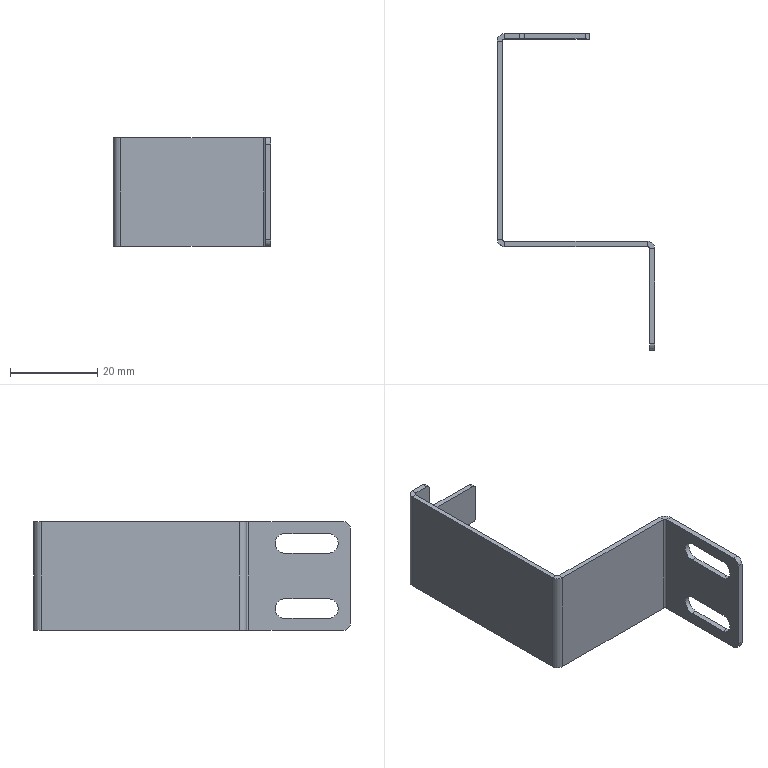Part | SolidWorks | features Fillet 2, FlatPattern 1, HoleWzd 1, ICE 1, SMBaseFlange 1, SheetMetal 1 | 1 solid | 48 faces | box 36.2 x 72.7 x 25 mm | volume 3370 mm3 | plane 32 | cylinder 16 | commonest cylinder face diameters 2 x4 4.5 x4 1 x3 3.4 x3 3 x2
STEP:
#1=CARTESIAN_POINT('',(0.,-20.,5.25));
#2=VERTEX_POINT('',#1);
#3=CARTESIAN_POINT('',(0.,-10.,5.25));
#4=VERTEX_POINT('',#3);
#5=CARTESIAN_POINT('',(0.,-20.,5.25));
#6=DIRECTION('',(0.,1.,0.));
#7=VECTOR('',#6,1000.);
#8=LINE('',#5,#7);
#9=EDGE_CURVE('',#2,#4,#8,.T.);
#10=ORIENTED_EDGE('',*,*,#9,.F.);
#11=CARTESIAN_POINT('',(0.,-20.,9.75));
#12=VERTEX_POINT('',#11);
#13=CARTESIAN_POINT('',(0.,-20.,7.5));
#14=DIRECTION('',(-1.,0.,0.));
#15=DIRECTION('',(0.,0.,1.));
#16=AXIS2_PLACEMENT_3D('',#13,#14,#15);
#17=CIRCLE('',#16,2.25);
#18=EDGE_CURVE('',#2,#12,#17,.T.);
#19=ORIENTED_EDGE('',*,*,#18,.T.);
#20=CARTESIAN_POINT('',(0.,-10.,9.75));
#21=VERTEX_POINT('',#20);
#22=CARTESIAN_POINT('',(0.,-20.,9.75));
#23=DIRECTION('',(0.,1.,0.));
#24=VECTOR('',#23,1000.);
#25=LINE('',#22,#24);
#26=EDGE_CURVE('',#12,#21,#25,.T.);
#27=ORIENTED_EDGE('',*,*,#26,.T.);
#28=CARTESIAN_POINT('',(0.,-10.,7.5));
#29=DIRECTION('',(-1.,0.,0.));
#30=DIRECTION('',(0.,0.,1.));
#31=AXIS2_PLACEMENT_3D('',#28,#29,#30);
#32=CIRCLE('',#31,2.25);
#33=EDGE_CURVE('',#21,#4,#32,.T.);
#34=ORIENTED_EDGE('',*,*,#33,.T.);
#35=EDGE_LOOP('',(#10,#19,#27,#34));
#36=FACE_BOUND('',#35,.T.);
#37=CARTESIAN_POINT('',(0.,-25.,11.));
#38=VERTEX_POINT('',#37);
#39=CARTESIAN_POINT('',(0.,-25.,-11.));
#40=VERTEX_POINT('',#39);
#41=CARTESIAN_POINT('',(0.,-25.,12.5));
#42=DIRECTION('',(0.,0.,-1.));
#43=VECTOR('',#42,1000.);
#44=LINE('',#41,#43);
#45=EDGE_CURVE('',#38,#40,#44,.T.);
#46=ORIENTED_EDGE('',*,*,#45,.T.);
#47=CARTESIAN_POINT('',(0.,-23.5,-12.5));
#48=VERTEX_POINT('',#47);
#49=CARTESIAN_POINT('',(0.,-23.5,-11.));
#50=DIRECTION('',(1.,0.,0.));
#51=DIRECTION('',(0.,0.,-1.));
#52=AXIS2_PLACEMENT_3D('',#49,#50,#51);
#53=CIRCLE('',#52,1.5);
#54=EDGE_CURVE('',#40,#48,#53,.T.);
#55=ORIENTED_EDGE('',*,*,#54,.T.);
#56=CARTESIAN_POINT('',(0.,-1.7,-12.5));
#57=VERTEX_POINT('',#56);
#58=CARTESIAN_POINT('',(0.,0.,-12.5));
#59=DIRECTION('',(0.,-1.,0.));
#60=VECTOR('',#59,1000.);
#61=LINE('',#58,#60);
#62=EDGE_CURVE('',#57,#48,#61,.T.);
#63=ORIENTED_EDGE('',*,*,#62,.F.);
#64=CARTESIAN_POINT('',(0.,-1.7,12.5));
#65=VERTEX_POINT('',#64);
#66=CARTESIAN_POINT('',(0.,-1.7,12.5));
#67=DIRECTION('',(0.,0.,-1.));
#68=VECTOR('',#67,1000.);
#69=LINE('',#66,#68);
#70=EDGE_CURVE('',#65,#57,#69,.T.);
#71=ORIENTED_EDGE('',*,*,#70,.F.);
#72=CARTESIAN_POINT('',(0.,-23.5,12.5));
#73=VERTEX_POINT('',#72);
#74=CARTESIAN_POINT('',(0.,0.,12.5));
#75=DIRECTION('',(0.,-1.,0.));
#76=VECTOR('',#75,1000.);
#77=LINE('',#74,#76);
#78=EDGE_CURVE('',#65,#73,#77,.T.);
#79=ORIENTED_EDGE('',*,*,#78,.T.);
#80=CARTESIAN_POINT('',(0.,-23.5,11.));
#81=DIRECTION('',(1.,0.,0.));
#82=DIRECTION('',(0.,0.,-1.));
#83=AXIS2_PLACEMENT_3D('',#80,#81,#82);
#84=CIRCLE('',#83,1.5);
#85=EDGE_CURVE('',#73,#38,#84,.T.);
#86=ORIENTED_EDGE('',*,*,#85,.T.);
#87=EDGE_LOOP('',(#46,#55,#63,#71,#79,#86));
#88=FACE_OUTER_BOUND('',#87,.T.);
#89=CARTESIAN_POINT('',(0.,-20.,-9.75));
#90=VERTEX_POINT('',#89);
#91=CARTESIAN_POINT('',(0.,-20.,-5.25));
#92=VERTEX_POINT('',#91);
#93=CARTESIAN_POINT('',(0.,-20.,-7.5));
#94=DIRECTION('',(-1.,0.,0.));
#95=DIRECTION('',(0.,0.,1.));
#96=AXIS2_PLACEMENT_3D('',#93,#94,#95);
#97=CIRCLE('',#96,2.25);
#98=EDGE_CURVE('',#90,#92,#97,.T.);
#99=ORIENTED_EDGE('',*,*,#98,.T.);
#100=CARTESIAN_POINT('',(0.,-10.,-5.25));
#101=VERTEX_POINT('',#100);
#102=CARTESIAN_POINT('',(0.,-20.,-5.25));
#103=DIRECTION('',(0.,1.,0.));
#104=VECTOR('',#103,1000.);
#105=LINE('',#102,#104);
#106=EDGE_CURVE('',#92,#101,#105,.T.);
#107=ORIENTED_EDGE('',*,*,#106,.T.);
#108=CARTESIAN_POINT('',(0.,-10.,-9.75));
#109=VERTEX_POINT('',#108);
#110=CARTESIAN_POINT('',(0.,-10.,-7.5));
#111=DIRECTION('',(-1.,0.,0.));
#112=DIRECTION('',(0.,0.,1.));
#113=AXIS2_PLACEMENT_3D('',#110,#111,#112);
#114=CIRCLE('',#113,2.25);
#115=EDGE_CURVE('',#101,#109,#114,.T.);
#116=ORIENTED_EDGE('',*,*,#115,.T.);
#117=CARTESIAN_POINT('',(0.,-20.,-9.75));
#118=DIRECTION('',(0.,1.,0.));
#119=VECTOR('',#118,1000.);
#120=LINE('',#117,#119);
#121=EDGE_CURVE('',#90,#109,#120,.T.);
#122=ORIENTED_EDGE('',*,*,#121,.F.);
#123=EDGE_LOOP('',(#99,#107,#116,#122));
#124=FACE_BOUND('',#123,.T.);
#125=CARTESIAN_POINT('',(0.,0.,12.5));
#126=DIRECTION('',(1.,0.,0.));
#127=DIRECTION('',(0.,0.,-1.));
#128=AXIS2_PLACEMENT_3D('',#125,#126,#127);
#129=PLANE('',#128);
#130=ADVANCED_FACE('',(#36,#88,#124),#129,.T.);
#131=CARTESIAN_POINT('',(-31.,47.7,-12.5));
#132=VERTEX_POINT('',#131);
#133=CARTESIAN_POINT('',(-34.5,47.7,-12.5));
#134=VERTEX_POINT('',#133);
#135=CARTESIAN_POINT('',(-35.,47.7,-12.5));
#136=DIRECTION('',(-1.,0.,0.));
#137=VECTOR('',#136,1000.);
#138=LINE('',#135,#137);
#139=EDGE_CURVE('',#132,#134,#138,.T.);
#140=ORIENTED_EDGE('',*,*,#139,.F.);
#141=CARTESIAN_POINT('',(-31.,46.5,-12.5));
#142=VERTEX_POINT('',#141);
#143=CARTESIAN_POINT('',(-31.,46.,-12.5));
#144=DIRECTION('',(0.,-1.,0.));
#145=VECTOR('',#144,1000.);
#146=LINE('',#143,#145);
#147=EDGE_CURVE('',#132,#142,#146,.T.);
#148=ORIENTED_EDGE('',*,*,#147,.T.);
#149=CARTESIAN_POINT('',(-34.5,46.5,-12.5));
#150=VERTEX_POINT('',#149);
#151=CARTESIAN_POINT('',(-35.,46.5,-12.5));
#152=DIRECTION('',(-1.,0.,0.));
#153=VECTOR('',#152,1000.);
#154=LINE('',#151,#153);
#155=EDGE_CURVE('',#142,#150,#154,.T.);
#156=ORIENTED_EDGE('',*,*,#155,.T.);
#157=CARTESIAN_POINT('',(-34.5,46.5,-12.5));
#158=DIRECTION('',(0.,1.,0.));
#159=VECTOR('',#158,1000.);
#160=LINE('',#157,#159);
#161=EDGE_CURVE('',#150,#134,#160,.T.);
#162=ORIENTED_EDGE('',*,*,#161,.T.);
#163=EDGE_LOOP('',(#140,#148,#156,#162));
#164=FACE_OUTER_BOUND('',#163,.T.);
#165=CARTESIAN_POINT('',(-36.2,46.,-12.5));
#166=DIRECTION('',(0.,0.,-1.));
#167=DIRECTION('',(-1.,0.,0.));
#168=AXIS2_PLACEMENT_3D('',#165,#166,#167);
#169=PLANE('',#168);
#170=ADVANCED_FACE('',(#164),#169,.T.);
#171=CARTESIAN_POINT('',(-30.,46.5,-5.));
#172=VERTEX_POINT('',#171);
#173=CARTESIAN_POINT('',(-16.,46.5,-5.));
#174=VERTEX_POINT('',#173);
#175=CARTESIAN_POINT('',(-30.,46.5,-5.));
#176=DIRECTION('',(1.,0.,0.));
#177=VECTOR('',#176,1000.);
#178=LINE('',#175,#177);
#179=EDGE_CURVE('',#172,#174,#178,.T.);
#180=ORIENTED_EDGE('',*,*,#179,.T.);
#181=CARTESIAN_POINT('',(-15.,46.5,-4.));
#182=VERTEX_POINT('',#181);
#183=CARTESIAN_POINT('',(-16.,46.5,-4.));
#184=DIRECTION('',(0.,-1.,0.));
#185=DIRECTION('',(0.,0.,-1.));
#186=AXIS2_PLACEMENT_3D('',#183,#184,#185);
#187=CIRCLE('',#186,1.);
#188=EDGE_CURVE('',#174,#182,#187,.T.);
#189=ORIENTED_EDGE('',*,*,#188,.T.);
#190=CARTESIAN_POINT('',(-15.,46.5,4.));
#191=VERTEX_POINT('',#190);
#192=CARTESIAN_POINT('',(-15.,46.5,12.5));
#193=DIRECTION('',(0.,0.,-1.));
#194=VECTOR('',#193,1000.);
#195=LINE('',#192,#194);
#196=EDGE_CURVE('',#191,#182,#195,.T.);
#197=ORIENTED_EDGE('',*,*,#196,.F.);
#198=CARTESIAN_POINT('',(-16.,46.5,5.));
#199=VERTEX_POINT('',#198);
#200=CARTESIAN_POINT('',(-16.,46.5,4.));
#201=DIRECTION('',(0.,-1.,0.));
#202=DIRECTION('',(0.,0.,-1.));
#203=AXIS2_PLACEMENT_3D('',#200,#201,#202);
#204=CIRCLE('',#203,1.);
#205=EDGE_CURVE('',#191,#199,#204,.T.);
#206=ORIENTED_EDGE('',*,*,#205,.T.);
#207=CARTESIAN_POINT('',(-30.,46.5,5.));
#208=VERTEX_POINT('',#207);
#209=CARTESIAN_POINT('',(-30.,46.5,5.));
#210=DIRECTION('',(-1.,0.,0.));
#211=VECTOR('',#210,1000.);
#212=LINE('',#209,#211);
#213=EDGE_CURVE('',#199,#208,#212,.T.);
#214=ORIENTED_EDGE('',*,*,#213,.T.);
#215=CARTESIAN_POINT('',(-30.,46.5,11.5));
#216=VERTEX_POINT('',#215);
#217=CARTESIAN_POINT('',(-30.,46.5,12.5));
#218=DIRECTION('',(0.,0.,1.));
#219=VECTOR('',#218,1000.);
#220=LINE('',#217,#219);
#221=EDGE_CURVE('',#208,#216,#220,.T.);
#222=ORIENTED_EDGE('',*,*,#221,.T.);
#223=CARTESIAN_POINT('',(-31.,46.5,12.5));
#224=VERTEX_POINT('',#223);
#225=CARTESIAN_POINT('',(-31.,46.5,11.5));
#226=DIRECTION('',(0.,-1.,0.));
#227=DIRECTION('',(0.,0.,-1.));
#228=AXIS2_PLACEMENT_3D('',#225,#226,#227);
#229=CIRCLE('',#228,1.);
#230=EDGE_CURVE('',#216,#224,#229,.T.);
#231=ORIENTED_EDGE('',*,*,#230,.T.);
#232=CARTESIAN_POINT('',(-34.5,46.5,12.5));
#233=VERTEX_POINT('',#232);
#234=CARTESIAN_POINT('',(-35.,46.5,12.5));
#235=DIRECTION('',(-1.,0.,0.));
#236=VECTOR('',#235,1000.);
#237=LINE('',#234,#236);
#238=EDGE_CURVE('',#224,#233,#237,.T.);
#239=ORIENTED_EDGE('',*,*,#238,.T.);
#240=CARTESIAN_POINT('',(-34.5,46.5,12.5));
#241=DIRECTION('',(0.,0.,-1.));
#242=VECTOR('',#241,1000.);
#243=LINE('',#240,#242);
#244=EDGE_CURVE('',#233,#150,#243,.T.);
#245=ORIENTED_EDGE('',*,*,#244,.T.);
#246=ORIENTED_EDGE('',*,*,#155,.F.);
#247=CARTESIAN_POINT('',(-30.,46.5,-11.5));
#248=VERTEX_POINT('',#247);
#249=CARTESIAN_POINT('',(-31.,46.5,-11.5));
#250=DIRECTION('',(0.,-1.,0.));
#251=DIRECTION('',(0.,0.,-1.));
#252=AXIS2_PLACEMENT_3D('',#249,#250,#251);
#253=CIRCLE('',#252,1.);
#254=EDGE_CURVE('',#142,#248,#253,.T.);
#255=ORIENTED_EDGE('',*,*,#254,.T.);
#256=CARTESIAN_POINT('',(-30.,46.5,-12.5));
#257=DIRECTION('',(0.,0.,1.));
#258=VECTOR('',#257,1000.);
#259=LINE('',#256,#258);
#260=EDGE_CURVE('',#248,#172,#259,.T.);
#261=ORIENTED_EDGE('',*,*,#260,.T.);
#262=EDGE_LOOP('',(#180,#189,#197,#206,#214,#222,#231,#239,#245,#246,#255,#261));
#263=FACE_OUTER_BOUND('',#262,.T.);
#264=CARTESIAN_POINT('',(-35.,46.5,12.5));
#265=DIRECTION('',(0.,-1.,0.));
#266=DIRECTION('',(0.,0.,-1.));
#267=AXIS2_PLACEMENT_3D('',#264,#265,#266);
#268=PLANE('',#267);
#269=ADVANCED_FACE('',(#263),#268,.T.);
#270=ORIENTED_EDGE('',*,*,#196,.T.);
#271=CARTESIAN_POINT('',(-15.,47.7,-4.));
#272=VERTEX_POINT('',#271);
#273=CARTESIAN_POINT('',(-15.,47.7,-4.));
#274=DIRECTION('',(0.,1.,0.));
#275=VECTOR('',#274,1000.);
#276=LINE('',#273,#275);
#277=EDGE_CURVE('',#182,#272,#276,.T.);
#278=ORIENTED_EDGE('',*,*,#277,.T.);
#279=CARTESIAN_POINT('',(-15.,47.7,4.));
#280=VERTEX_POINT('',#279);
#281=CARTESIAN_POINT('',(-15.,47.7,12.5));
#282=DIRECTION('',(0.,0.,-1.));
#283=VECTOR('',#282,1000.);
#284=LINE('',#281,#283);
#285=EDGE_CURVE('',#280,#272,#284,.T.);
#286=ORIENTED_EDGE('',*,*,#285,.F.);
#287=CARTESIAN_POINT('',(-15.,47.7,4.));
#288=DIRECTION('',(0.,-1.,0.));
#289=VECTOR('',#288,1000.);
#290=LINE('',#287,#289);
#291=EDGE_CURVE('',#280,#191,#290,.T.);
#292=ORIENTED_EDGE('',*,*,#291,.T.);
#293=EDGE_LOOP('',(#270,#278,#286,#292));
#294=FACE_OUTER_BOUND('',#293,.T.);
#295=CARTESIAN_POINT('',(-15.,47.7,12.5));
#296=DIRECTION('',(1.,0.,0.));
#297=DIRECTION('',(0.,1.,0.));
#298=AXIS2_PLACEMENT_3D('',#295,#296,#297);
#299=PLANE('',#298);
#300=ADVANCED_FACE('',(#294),#299,.T.);
#301=ORIENTED_EDGE('',*,*,#285,.T.);
#302=CARTESIAN_POINT('',(-16.,47.7,-5.));
#303=VERTEX_POINT('',#302);
#304=CARTESIAN_POINT('',(-16.,47.7,-4.));
#305=DIRECTION('',(0.,1.,0.));
#306=DIRECTION('',(0.,0.,-1.));
#307=AXIS2_PLACEMENT_3D('',#304,#305,#306);
#308=CIRCLE('',#307,1.);
#309=EDGE_CURVE('',#272,#303,#308,.T.);
#310=ORIENTED_EDGE('',*,*,#309,.T.);
#311=CARTESIAN_POINT('',(-30.,47.7,-5.));
#312=VERTEX_POINT('',#311);
#313=CARTESIAN_POINT('',(-30.,47.7,-5.));
#314=DIRECTION('',(-1.,0.,0.));
#315=VECTOR('',#314,1000.);
#316=LINE('',#313,#315);
#317=EDGE_CURVE('',#303,#312,#316,.T.);
#318=ORIENTED_EDGE('',*,*,#317,.T.);
#319=CARTESIAN_POINT('',(-30.,47.7,-11.5));
#320=VERTEX_POINT('',#319);
#321=CARTESIAN_POINT('',(-30.,47.7,-12.5));
#322=DIRECTION('',(0.,0.,-1.));
#323=VECTOR('',#322,1000.);
#324=LINE('',#321,#323);
#325=EDGE_CURVE('',#312,#320,#324,.T.);
#326=ORIENTED_EDGE('',*,*,#325,.T.);
#327=CARTESIAN_POINT('',(-31.,47.7,-11.5));
#328=DIRECTION('',(0.,1.,0.));
#329=DIRECTION('',(0.,0.,-1.));
#330=AXIS2_PLACEMENT_3D('',#327,#328,#329);
#331=CIRCLE('',#330,1.);
#332=EDGE_CURVE('',#320,#132,#331,.T.);
#333=ORIENTED_EDGE('',*,*,#332,.T.);
#334=ORIENTED_EDGE('',*,*,#139,.T.);
#335=CARTESIAN_POINT('',(-34.5,47.7,12.5));
#336=VERTEX_POINT('',#335);
#337=CARTESIAN_POINT('',(-34.5,47.7,12.5));
#338=DIRECTION('',(0.,0.,-1.));
#339=VECTOR('',#338,1000.);
#340=LINE('',#337,#339);
#341=EDGE_CURVE('',#336,#134,#340,.T.);
#342=ORIENTED_EDGE('',*,*,#341,.F.);
#343=CARTESIAN_POINT('',(-31.,47.7,12.5));
#344=VERTEX_POINT('',#343);
#345=CARTESIAN_POINT('',(-35.,47.7,12.5));
#346=DIRECTION('',(-1.,0.,0.));
#347=VECTOR('',#346,1000.);
#348=LINE('',#345,#347);
#349=EDGE_CURVE('',#344,#336,#348,.T.);
#350=ORIENTED_EDGE('',*,*,#349,.F.);
#351=CARTESIAN_POINT('',(-30.,47.7,11.5));
#352=VERTEX_POINT('',#351);
#353=CARTESIAN_POINT('',(-31.,47.7,11.5));
#354=DIRECTION('',(0.,1.,0.));
#355=DIRECTION('',(0.,0.,-1.));
#356=AXIS2_PLACEMENT_3D('',#353,#354,#355);
#357=CIRCLE('',#356,1.);
#358=EDGE_CURVE('',#344,#352,#357,.T.);
#359=ORIENTED_EDGE('',*,*,#358,.T.);
#360=CARTESIAN_POINT('',(-30.,47.7,5.));
#361=VERTEX_POINT('',#360);
#362=CARTESIAN_POINT('',(-30.,47.7,12.5));
#363=DIRECTION('',(0.,0.,-1.));
#364=VECTOR('',#363,1000.);
#365=LINE('',#362,#364);
#366=EDGE_CURVE('',#352,#361,#365,.T.);
#367=ORIENTED_EDGE('',*,*,#366,.T.);
#368=CARTESIAN_POINT('',(-16.,47.7,5.));
#369=VERTEX_POINT('',#368);
#370=CARTESIAN_POINT('',(-30.,47.7,5.));
#371=DIRECTION('',(1.,0.,0.));
#372=VECTOR('',#371,1000.);
#373=LINE('',#370,#372);
#374=EDGE_CURVE('',#361,#369,#373,.T.);
#375=ORIENTED_EDGE('',*,*,#374,.T.);
#376=CARTESIAN_POINT('',(-16.,47.7,4.));
#377=DIRECTION('',(0.,1.,0.));
#378=DIRECTION('',(0.,0.,-1.));
#379=AXIS2_PLACEMENT_3D('',#376,#377,#378);
#380=CIRCLE('',#379,1.);
#381=EDGE_CURVE('',#369,#280,#380,.T.);
#382=ORIENTED_EDGE('',*,*,#381,.T.);
#383=EDGE_LOOP('',(#301,#310,#318,#326,#333,#334,#342,#350,#359,#367,#375,#382));
#384=FACE_OUTER_BOUND('',#383,.T.);
#385=CARTESIAN_POINT('',(-35.,47.7,12.5));
#386=DIRECTION('',(0.,-1.,0.));
#387=DIRECTION('',(0.,0.,-1.));
#388=AXIS2_PLACEMENT_3D('',#385,#386,#387);
#389=PLANE('',#388);
#390=ADVANCED_FACE('',(#384),#389,.F.);
#391=ORIENTED_EDGE('',*,*,#238,.F.);
#392=CARTESIAN_POINT('',(-31.,47.7,12.5));
#393=DIRECTION('',(0.,1.,0.));
#394=VECTOR('',#393,1000.);
#395=LINE('',#392,#394);
#396=EDGE_CURVE('',#224,#344,#395,.T.);
#397=ORIENTED_EDGE('',*,*,#396,.T.);
#398=ORIENTED_EDGE('',*,*,#349,.T.);
#399=CARTESIAN_POINT('',(-34.5,47.7,12.5));
#400=DIRECTION('',(0.,-1.,0.));
#401=VECTOR('',#400,1000.);
#402=LINE('',#399,#401);
#403=EDGE_CURVE('',#336,#233,#402,.T.);
#404=ORIENTED_EDGE('',*,*,#403,.T.);
#405=EDGE_LOOP('',(#391,#397,#398,#404));
#406=FACE_OUTER_BOUND('',#405,.T.);
#407=CARTESIAN_POINT('',(-1.7,-1.7,12.5));
#408=DIRECTION('',(0.,0.,-1.));
#409=DIRECTION('',(-1.,0.,0.));
#410=AXIS2_PLACEMENT_3D('',#407,#408,#409);
#411=PLANE('',#410);
#412=ADVANCED_FACE('',(#406),#411,.F.);
#413=CARTESIAN_POINT('',(-1.2,-1.7,12.5));
#414=VERTEX_POINT('',#413);
#415=CARTESIAN_POINT('',(0.,-1.7,12.5));
#416=DIRECTION('',(-1.,0.,0.));
#417=VECTOR('',#416,1000.);
#418=LINE('',#415,#417);
#419=EDGE_CURVE('',#65,#414,#418,.T.);
#420=ORIENTED_EDGE('',*,*,#419,.F.);
#421=CARTESIAN_POINT('',(-1.7,0.,12.5));
#422=VERTEX_POINT('',#421);
#423=CARTESIAN_POINT('',(-1.7,-1.7,12.5));
#424=DIRECTION('',(0.,0.,-1.));
#425=DIRECTION('',(-1.,0.,0.));
#426=AXIS2_PLACEMENT_3D('',#423,#424,#425);
#427=CIRCLE('',#426,1.7);
#428=EDGE_CURVE('',#422,#65,#427,.T.);
#429=ORIENTED_EDGE('',*,*,#428,.F.);
#430=CARTESIAN_POINT('',(-1.7,-1.2,12.5));
#431=VERTEX_POINT('',#430);
#432=CARTESIAN_POINT('',(-1.7,-1.2,12.5));
#433=DIRECTION('',(0.,1.,0.));
#434=VECTOR('',#433,1000.);
#435=LINE('',#432,#434);
#436=EDGE_CURVE('',#431,#422,#435,.T.);
#437=ORIENTED_EDGE('',*,*,#436,.F.);
#438=CARTESIAN_POINT('',(-1.7,-1.7,12.5));
#439=DIRECTION('',(0.,0.,-1.));
#440=DIRECTION('',(1.,0.,0.));
#441=AXIS2_PLACEMENT_3D('',#438,#439,#440);
#442=CIRCLE('',#441,0.5);
#443=EDGE_CURVE('',#431,#414,#442,.T.);
#444=ORIENTED_EDGE('',*,*,#443,.T.);
#445=EDGE_LOOP('',(#420,#429,#437,#444));
#446=FACE_OUTER_BOUND('',#445,.T.);
#447=CARTESIAN_POINT('',(0.,-1.7,12.5));
#448=DIRECTION('',(0.,0.,1.));
#449=DIRECTION('',(1.,0.,0.));
#450=AXIS2_PLACEMENT_3D('',#447,#448,#449);
#451=PLANE('',#450);
#452=ADVANCED_FACE('',(#446),#451,.T.);
#453=CARTESIAN_POINT('',(-1.2,-23.5,12.5));
#454=VERTEX_POINT('',#453);
#455=CARTESIAN_POINT('',(-1.2,0.,12.5));
#456=DIRECTION('',(0.,-1.,0.));
#457=VECTOR('',#456,1000.);
#458=LINE('',#455,#457);
#459=EDGE_CURVE('',#414,#454,#458,.T.);
#460=ORIENTED_EDGE('',*,*,#459,.T.);
#461=CARTESIAN_POINT('',(-1.7,-23.5,12.5));
#462=DIRECTION('',(1.,0.,0.));
#463=VECTOR('',#462,1000.);
#464=LINE('',#461,#463);
#465=EDGE_CURVE('',#454,#73,#464,.T.);
#466=ORIENTED_EDGE('',*,*,#465,.T.);
#467=ORIENTED_EDGE('',*,*,#78,.F.);
#468=ORIENTED_EDGE('',*,*,#419,.T.);
#469=EDGE_LOOP('',(#460,#466,#467,#468));
#470=FACE_OUTER_BOUND('',#469,.T.);
#471=CARTESIAN_POINT('',(-1.7,-1.2,12.5));
#472=DIRECTION('',(0.,0.,1.));
#473=DIRECTION('',(1.,0.,0.));
#474=AXIS2_PLACEMENT_3D('',#471,#472,#473);
#475=PLANE('',#474);
#476=ADVANCED_FACE('',(#470),#475,.T.);
#477=CARTESIAN_POINT('',(-1.7,0.,-12.5));
#478=VERTEX_POINT('',#477);
#479=CARTESIAN_POINT('',(-1.7,-1.2,-12.5));
#480=VERTEX_POINT('',#479);
#481=CARTESIAN_POINT('',(-1.7,0.,-12.5));
#482=DIRECTION('',(0.,-1.,0.));
#483=VECTOR('',#482,1000.);
#484=LINE('',#481,#483);
#485=EDGE_CURVE('',#478,#480,#484,.T.);
#486=ORIENTED_EDGE('',*,*,#485,.F.);
#487=CARTESIAN_POINT('',(-1.7,-1.7,-12.5));
#488=DIRECTION('',(0.,0.,-1.));
#489=DIRECTION('',(-1.,0.,0.));
#490=AXIS2_PLACEMENT_3D('',#487,#488,#489);
#491=CIRCLE('',#490,1.7);
#492=EDGE_CURVE('',#478,#57,#491,.T.);
#493=ORIENTED_EDGE('',*,*,#492,.T.);
#494=CARTESIAN_POINT('',(-1.2,-1.7,-12.5));
#495=VERTEX_POINT('',#494);
#496=CARTESIAN_POINT('',(-1.2,-1.7,-12.5));
#497=DIRECTION('',(1.,0.,0.));
#498=VECTOR('',#497,1000.);
#499=LINE('',#496,#498);
#500=EDGE_CURVE('',#495,#57,#499,.T.);
#501=ORIENTED_EDGE('',*,*,#500,.F.);
#502=CARTESIAN_POINT('',(-1.7,-1.7,-12.5));
#503=DIRECTION('',(0.,0.,-1.));
#504=DIRECTION('',(1.,0.,0.));
#505=AXIS2_PLACEMENT_3D('',#502,#503,#504);
#506=CIRCLE('',#505,0.5);
#507=EDGE_CURVE('',#480,#495,#506,.T.);
#508=ORIENTED_EDGE('',*,*,#507,.F.);
#509=EDGE_LOOP('',(#486,#493,#501,#508));
#510=FACE_OUTER_BOUND('',#509,.T.);
#511=CARTESIAN_POINT('',(-1.7,0.,-12.5));
#512=DIRECTION('',(0.,0.,-1.));
#513=DIRECTION('',(-1.,0.,0.));
#514=AXIS2_PLACEMENT_3D('',#511,#512,#513);
#515=PLANE('',#514);
#516=ADVANCED_FACE('',(#510),#515,.T.);
#517=CARTESIAN_POINT('',(-34.5,0.,-12.5));
#518=VERTEX_POINT('',#517);
#519=CARTESIAN_POINT('',(-35.,0.,-12.5));
#520=DIRECTION('',(1.,0.,0.));
#521=VECTOR('',#520,1000.);
#522=LINE('',#519,#521);
#523=EDGE_CURVE('',#518,#478,#522,.T.);
#524=ORIENTED_EDGE('',*,*,#523,.T.);
#525=ORIENTED_EDGE('',*,*,#485,.T.);
#526=CARTESIAN_POINT('',(-34.5,-1.2,-12.5));
#527=VERTEX_POINT('',#526);
#528=CARTESIAN_POINT('',(-35.,-1.2,-12.5));
#529=DIRECTION('',(1.,0.,0.));
#530=VECTOR('',#529,1000.);
#531=LINE('',#528,#530);
#532=EDGE_CURVE('',#527,#480,#531,.T.);
#533=ORIENTED_EDGE('',*,*,#532,.F.);
#534=CARTESIAN_POINT('',(-34.5,-1.2,-12.5));
#535=DIRECTION('',(0.,1.,0.));
#536=VECTOR('',#535,1000.);
#537=LINE('',#534,#536);
#538=EDGE_CURVE('',#527,#518,#537,.T.);
#539=ORIENTED_EDGE('',*,*,#538,.T.);
#540=EDGE_LOOP('',(#524,#525,#533,#539));
#541=FACE_OUTER_BOUND('',#540,.T.);
#542=CARTESIAN_POINT('',(-1.2,-1.7,-12.5));
#543=DIRECTION('',(0.,0.,-1.));
#544=DIRECTION('',(-1.,0.,0.));
#545=AXIS2_PLACEMENT_3D('',#542,#543,#544);
#546=PLANE('',#545);
#547=ADVANCED_FACE('',(#541),#546,.T.);
#548=CARTESIAN_POINT('',(-34.5,0.,12.5));
#549=VERTEX_POINT('',#548);
#550=CARTESIAN_POINT('',(-34.5,-1.2,12.5));
#551=VERTEX_POINT('',#550);
#552=CARTESIAN_POINT('',(-34.5,0.,12.5));
#553=DIRECTION('',(0.,-1.,0.));
#554=VECTOR('',#553,1000.);
#555=LINE('',#552,#554);
#556=EDGE_CURVE('',#549,#551,#555,.T.);
#557=ORIENTED_EDGE('',*,*,#556,.F.);
#558=CARTESIAN_POINT('',(-35.,0.5,12.5));
#559=VERTEX_POINT('',#558);
#560=CARTESIAN_POINT('',(-34.5,0.5,12.5));
#561=DIRECTION('',(0.,0.,1.));
#562=DIRECTION('',(1.,0.,0.));
#563=AXIS2_PLACEMENT_3D('',#560,#561,#562);
#564=CIRCLE('',#563,0.5);
#565=EDGE_CURVE('',#559,#549,#564,.T.);
#566=ORIENTED_EDGE('',*,*,#565,.F.);
#567=CARTESIAN_POINT('',(-36.2,0.5,12.5));
#568=VERTEX_POINT('',#567);
#569=CARTESIAN_POINT('',(-36.2,0.5,12.5));
#570=DIRECTION('',(1.,0.,0.));
#571=VECTOR('',#570,1000.);
#572=LINE('',#569,#571);
#573=EDGE_CURVE('',#568,#559,#572,.T.);
#574=ORIENTED_EDGE('',*,*,#573,.F.);
#575=CARTESIAN_POINT('',(-34.5,0.5,12.5));
#576=DIRECTION('',(0.,0.,1.));
#577=DIRECTION('',(1.,0.,0.));
#578=AXIS2_PLACEMENT_3D('',#575,#576,#577);
#579=CIRCLE('',#578,1.7);
#580=EDGE_CURVE('',#568,#551,#579,.T.);
#581=ORIENTED_EDGE('',*,*,#580,.T.);
#582=EDGE_LOOP('',(#557,#566,#574,#581));
#583=FACE_OUTER_BOUND('',#582,.T.);
#584=CARTESIAN_POINT('',(-34.5,0.,12.5));
#585=DIRECTION('',(0.,0.,1.));
#586=DIRECTION('',(1.,0.,0.));
#587=AXIS2_PLACEMENT_3D('',#584,#585,#586);
#588=PLANE('',#587);
#589=ADVANCED_FACE('',(#583),#588,.T.);
#590=CARTESIAN_POINT('',(-35.,0.,12.5));
#591=DIRECTION('',(1.,0.,0.));
#592=VECTOR('',#591,1000.);
#593=LINE('',#590,#592);
#594=EDGE_CURVE('',#549,#422,#593,.T.);
#595=ORIENTED_EDGE('',*,*,#594,.F.);
#596=ORIENTED_EDGE('',*,*,#556,.T.);
#597=CARTESIAN_POINT('',(-35.,-1.2,12.5));
#598=DIRECTION('',(1.,0.,0.));
#599=VECTOR('',#598,1000.);
#600=LINE('',#597,#599);
#601=EDGE_CURVE('',#551,#431,#600,.T.);
#602=ORIENTED_EDGE('',*,*,#601,.T.);
#603=ORIENTED_EDGE('',*,*,#436,.T.);
#604=EDGE_LOOP('',(#595,#596,#602,#603));
#605=FACE_OUTER_BOUND('',#604,.T.);
#606=CARTESIAN_POINT('',(-36.2,0.5,12.5));
#607=DIRECTION('',(0.,0.,1.));
#608=DIRECTION('',(1.,0.,0.));
#609=AXIS2_PLACEMENT_3D('',#606,#607,#608);
#610=PLANE('',#609);
#611=ADVANCED_FACE('',(#605),#610,.T.);
#612=CARTESIAN_POINT('',(-35.,0.5,-12.5));
#613=VERTEX_POINT('',#612);
#614=CARTESIAN_POINT('',(-36.2,0.5,-12.5));
#615=VERTEX_POINT('',#614);
#616=CARTESIAN_POINT('',(-35.,0.5,-12.5));
#617=DIRECTION('',(-1.,0.,0.));
#618=VECTOR('',#617,1000.);
#619=LINE('',#616,#618);
#620=EDGE_CURVE('',#613,#615,#619,.T.);
#621=ORIENTED_EDGE('',*,*,#620,.F.);
#622=CARTESIAN_POINT('',(-34.5,0.5,-12.5));
#623=DIRECTION('',(0.,0.,1.));
#624=DIRECTION('',(1.,0.,0.));
#625=AXIS2_PLACEMENT_3D('',#622,#623,#624);
#626=CIRCLE('',#625,0.5);
#627=EDGE_CURVE('',#613,#518,#626,.T.);
#628=ORIENTED_EDGE('',*,*,#627,.T.);
#629=ORIENTED_EDGE('',*,*,#538,.F.);
#630=CARTESIAN_POINT('',(-34.5,0.5,-12.5));
#631=DIRECTION('',(0.,0.,1.));
#632=DIRECTION('',(1.,0.,0.));
#633=AXIS2_PLACEMENT_3D('',#630,#631,#632);
#634=CIRCLE('',#633,1.7);
#635=EDGE_CURVE('',#615,#527,#634,.T.);
#636=ORIENTED_EDGE('',*,*,#635,.F.);
#637=EDGE_LOOP('',(#621,#628,#629,#636));
#638=FACE_OUTER_BOUND('',#637,.T.);
#639=CARTESIAN_POINT('',(-35.,0.5,-12.5));
#640=DIRECTION('',(0.,0.,-1.));
#641=DIRECTION('',(-1.,0.,0.));
#642=AXIS2_PLACEMENT_3D('',#639,#640,#641);
#643=PLANE('',#642);
#644=ADVANCED_FACE('',(#638),#643,.T.);
#645=CARTESIAN_POINT('',(-35.,46.,-12.5));
#646=VERTEX_POINT('',#645);
#647=CARTESIAN_POINT('',(-35.,0.,-12.5));
#648=DIRECTION('',(0.,-1.,0.));
#649=VECTOR('',#648,1000.);
#650=LINE('',#647,#649);
#651=EDGE_CURVE('',#646,#613,#650,.T.);
#652=ORIENTED_EDGE('',*,*,#651,.T.);
#653=ORIENTED_EDGE('',*,*,#620,.T.);
#654=CARTESIAN_POINT('',(-36.2,46.,-12.5));
#655=VERTEX_POINT('',#654);
#656=CARTESIAN_POINT('',(-36.2,0.,-12.5));
#657=DIRECTION('',(0.,-1.,0.));
#658=VECTOR('',#657,1000.);
#659=LINE('',#656,#658);
#660=EDGE_CURVE('',#655,#615,#659,.T.);
#661=ORIENTED_EDGE('',*,*,#660,.F.);
#662=CARTESIAN_POINT('',(-36.2,46.,-12.5));
#663=DIRECTION('',(1.,0.,0.));
#664=VECTOR('',#663,1000.);
#665=LINE('',#662,#664);
#666=EDGE_CURVE('',#655,#646,#665,.T.);
#667=ORIENTED_EDGE('',*,*,#666,.T.);
#668=EDGE_LOOP('',(#652,#653,#661,#667));
#669=FACE_OUTER_BOUND('',#668,.T.);
#670=CARTESIAN_POINT('',(-34.5,-1.2,-12.5));
#671=DIRECTION('',(0.,0.,-1.));
#672=DIRECTION('',(-1.,0.,0.));
#673=AXIS2_PLACEMENT_3D('',#670,#671,#672);
#674=PLANE('',#673);
#675=ADVANCED_FACE('',(#669),#674,.T.);
#676=CARTESIAN_POINT('',(-35.,46.,12.5));
#677=VERTEX_POINT('',#676);
#678=CARTESIAN_POINT('',(-36.2,46.,12.5));
#679=VERTEX_POINT('',#678);
#680=CARTESIAN_POINT('',(-35.,46.,12.5));
#681=DIRECTION('',(-1.,0.,0.));
#682=VECTOR('',#681,1000.);
#683=LINE('',#680,#682);
#684=EDGE_CURVE('',#677,#679,#683,.T.);
#685=ORIENTED_EDGE('',*,*,#684,.F.);
#686=CARTESIAN_POINT('',(-34.5,46.,12.5));
#687=DIRECTION('',(0.,0.,1.));
#688=DIRECTION('',(1.,0.,0.));
#689=AXIS2_PLACEMENT_3D('',#686,#687,#688);
#690=CIRCLE('',#689,0.5);
#691=EDGE_CURVE('',#233,#677,#690,.T.);
#692=ORIENTED_EDGE('',*,*,#691,.F.);
#693=ORIENTED_EDGE('',*,*,#403,.F.);
#694=CARTESIAN_POINT('',(-34.5,46.,12.5));
#695=DIRECTION('',(0.,0.,1.));
#696=DIRECTION('',(1.,0.,0.));
#697=AXIS2_PLACEMENT_3D('',#694,#695,#696);
#698=CIRCLE('',#697,1.7);
#699=EDGE_CURVE('',#336,#679,#698,.T.);
#700=ORIENTED_EDGE('',*,*,#699,.T.);
#701=EDGE_LOOP('',(#685,#692,#693,#700));
#702=FACE_OUTER_BOUND('',#701,.T.);
#703=CARTESIAN_POINT('',(-35.,46.,12.5));
#704=DIRECTION('',(0.,0.,1.));
#705=DIRECTION('',(1.,0.,0.));
#706=AXIS2_PLACEMENT_3D('',#703,#704,#705);
#707=PLANE('',#706);
#708=ADVANCED_FACE('',(#702),#707,.T.);
#709=CARTESIAN_POINT('',(-35.,0.,12.5));
#710=DIRECTION('',(0.,-1.,0.));
#711=VECTOR('',#710,1000.);
#712=LINE('',#709,#711);
#713=EDGE_CURVE('',#677,#559,#712,.T.);
#714=ORIENTED_EDGE('',*,*,#713,.F.);
#715=ORIENTED_EDGE('',*,*,#684,.T.);
#716=CARTESIAN_POINT('',(-36.2,0.,12.5));
#717=DIRECTION('',(0.,-1.,0.));
#718=VECTOR('',#717,1000.);
#719=LINE('',#716,#718);
#720=EDGE_CURVE('',#679,#568,#719,.T.);
#721=ORIENTED_EDGE('',*,*,#720,.T.);
#722=ORIENTED_EDGE('',*,*,#573,.T.);
#723=EDGE_LOOP('',(#714,#715,#721,#722));
#724=FACE_OUTER_BOUND('',#723,.T.);
#725=CARTESIAN_POINT('',(-34.5,47.7,12.5));
#726=DIRECTION('',(0.,0.,1.));
#727=DIRECTION('',(1.,0.,0.));
#728=AXIS2_PLACEMENT_3D('',#725,#726,#727);
#729=PLANE('',#728);
#730=ADVANCED_FACE('',(#724),#729,.T.);
#731=ORIENTED_EDGE('',*,*,#161,.F.);
#732=CARTESIAN_POINT('',(-34.5,46.,-12.5));
#733=DIRECTION('',(0.,0.,1.));
#734=DIRECTION('',(1.,0.,0.));
#735=AXIS2_PLACEMENT_3D('',#732,#733,#734);
#736=CIRCLE('',#735,0.5);
#737=EDGE_CURVE('',#150,#646,#736,.T.);
#738=ORIENTED_EDGE('',*,*,#737,.T.);
#739=ORIENTED_EDGE('',*,*,#666,.F.);
#740=CARTESIAN_POINT('',(-34.5,46.,-12.5));
#741=DIRECTION('',(0.,0.,1.));
#742=DIRECTION('',(1.,0.,0.));
#743=AXIS2_PLACEMENT_3D('',#740,#741,#742);
#744=CIRCLE('',#743,1.7);
#745=EDGE_CURVE('',#134,#655,#744,.T.);
#746=ORIENTED_EDGE('',*,*,#745,.F.);
#747=EDGE_LOOP('',(#731,#738,#739,#746));
#748=FACE_OUTER_BOUND('',#747,.T.);
#749=CARTESIAN_POINT('',(-34.5,46.5,-12.5));
#750=DIRECTION('',(0.,0.,-1.));
#751=DIRECTION('',(-1.,0.,0.));
#752=AXIS2_PLACEMENT_3D('',#749,#750,#751);
#753=PLANE('',#752);
#754=ADVANCED_FACE('',(#748),#753,.T.);
#755=CARTESIAN_POINT('',(-1.2,-20.,5.25));
#756=VERTEX_POINT('',#755);
#757=CARTESIAN_POINT('',(-1.2,-20.,9.75));
#758=VERTEX_POINT('',#757);
#759=CARTESIAN_POINT('',(-1.2,-20.,7.5));
#760=DIRECTION('',(-1.,0.,0.));
#761=DIRECTION('',(0.,0.,1.));
#762=AXIS2_PLACEMENT_3D('',#759,#760,#761);
#763=CIRCLE('',#762,2.25);
#764=EDGE_CURVE('',#756,#758,#763,.T.);
#765=ORIENTED_EDGE('',*,*,#764,.F.);
#766=CARTESIAN_POINT('',(-1.2,-10.,5.25));
#767=VERTEX_POINT('',#766);
#768=CARTESIAN_POINT('',(-1.2,-20.,5.25));
#769=DIRECTION('',(0.,1.,0.));
#770=VECTOR('',#769,1000.);
#771=LINE('',#768,#770);
#772=EDGE_CURVE('',#756,#767,#771,.T.);
#773=ORIENTED_EDGE('',*,*,#772,.T.);
#774=CARTESIAN_POINT('',(-1.2,-10.,9.75));
#775=VERTEX_POINT('',#774);
#776=CARTESIAN_POINT('',(-1.2,-10.,7.5));
#777=DIRECTION('',(-1.,0.,0.));
#778=DIRECTION('',(0.,0.,1.));
#779=AXIS2_PLACEMENT_3D('',#776,#777,#778);
#780=CIRCLE('',#779,2.25);
#781=EDGE_CURVE('',#775,#767,#780,.T.);
#782=ORIENTED_EDGE('',*,*,#781,.F.);
#783=CARTESIAN_POINT('',(-1.2,-20.,9.75));
#784=DIRECTION('',(0.,1.,0.));
#785=VECTOR('',#784,1000.);
#786=LINE('',#783,#785);
#787=EDGE_CURVE('',#758,#775,#786,.T.);
#788=ORIENTED_EDGE('',*,*,#787,.F.);
#789=EDGE_LOOP('',(#765,#773,#782,#788));
#790=FACE_BOUND('',#789,.T.);
#791=CARTESIAN_POINT('',(-1.2,-20.,-9.75));
#792=VERTEX_POINT('',#791);
#793=CARTESIAN_POINT('',(-1.2,-20.,-5.25));
#794=VERTEX_POINT('',#793);
#795=CARTESIAN_POINT('',(-1.2,-20.,-7.5));
#796=DIRECTION('',(-1.,0.,0.));
#797=DIRECTION('',(0.,0.,1.));
#798=AXIS2_PLACEMENT_3D('',#795,#796,#797);
#799=CIRCLE('',#798,2.25);
#800=EDGE_CURVE('',#792,#794,#799,.T.);
#801=ORIENTED_EDGE('',*,*,#800,.F.);
#802=CARTESIAN_POINT('',(-1.2,-10.,-9.75));
#803=VERTEX_POINT('',#802);
#804=CARTESIAN_POINT('',(-1.2,-20.,-9.75));
#805=DIRECTION('',(0.,1.,0.));
#806=VECTOR('',#805,1000.);
#807=LINE('',#804,#806);
#808=EDGE_CURVE('',#792,#803,#807,.T.);
#809=ORIENTED_EDGE('',*,*,#808,.T.);
#810=CARTESIAN_POINT('',(-1.2,-10.,-5.25));
#811=VERTEX_POINT('',#810);
#812=CARTESIAN_POINT('',(-1.2,-10.,-7.5));
#813=DIRECTION('',(-1.,0.,0.));
#814=DIRECTION('',(0.,0.,1.));
#815=AXIS2_PLACEMENT_3D('',#812,#813,#814);
#816=CIRCLE('',#815,2.25);
#817=EDGE_CURVE('',#811,#803,#816,.T.);
#818=ORIENTED_EDGE('',*,*,#817,.F.);
#819=CARTESIAN_POINT('',(-1.2,-20.,-5.25));
#820=DIRECTION('',(0.,1.,0.));
#821=VECTOR('',#820,1000.);
#822=LINE('',#819,#821);
#823=EDGE_CURVE('',#794,#811,#822,.T.);
#824=ORIENTED_EDGE('',*,*,#823,.F.);
#825=EDGE_LOOP('',(#801,#809,#818,#824));
#826=FACE_BOUND('',#825,.T.);
#827=CARTESIAN_POINT('',(-1.2,-23.5,-12.5));
#828=VERTEX_POINT('',#827);
#829=CARTESIAN_POINT('',(-1.2,0.,-12.5));
#830=DIRECTION('',(0.,-1.,0.));
#831=VECTOR('',#830,1000.);
#832=LINE('',#829,#831);
#833=EDGE_CURVE('',#495,#828,#832,.T.);
#834=ORIENTED_EDGE('',*,*,#833,.T.);
#835=CARTESIAN_POINT('',(-1.2,-25.,-11.));
#836=VERTEX_POINT('',#835);
#837=CARTESIAN_POINT('',(-1.2,-23.5,-11.));
#838=DIRECTION('',(-1.,0.,0.));
#839=DIRECTION('',(0.,0.,-1.));
#840=AXIS2_PLACEMENT_3D('',#837,#838,#839);
#841=CIRCLE('',#840,1.5);
#842=EDGE_CURVE('',#828,#836,#841,.T.);
#843=ORIENTED_EDGE('',*,*,#842,.T.);
#844=CARTESIAN_POINT('',(-1.2,-25.,11.));
#845=VERTEX_POINT('',#844);
#846=CARTESIAN_POINT('',(-1.2,-25.,12.5));
#847=DIRECTION('',(0.,0.,-1.));
#848=VECTOR('',#847,1000.);
#849=LINE('',#846,#848);
#850=EDGE_CURVE('',#845,#836,#849,.T.);
#851=ORIENTED_EDGE('',*,*,#850,.F.);
#852=CARTESIAN_POINT('',(-1.2,-23.5,11.));
#853=DIRECTION('',(-1.,0.,0.));
#854=DIRECTION('',(0.,0.,-1.));
#855=AXIS2_PLACEMENT_3D('',#852,#853,#854);
#856=CIRCLE('',#855,1.5);
#857=EDGE_CURVE('',#845,#454,#856,.T.);
#858=ORIENTED_EDGE('',*,*,#857,.T.);
#859=ORIENTED_EDGE('',*,*,#459,.F.);
#860=CARTESIAN_POINT('',(-1.2,-1.7,12.5));
#861=DIRECTION('',(0.,0.,-1.));
#862=VECTOR('',#861,1000.);
#863=LINE('',#860,#862);
#864=EDGE_CURVE('',#414,#495,#863,.T.);
#865=ORIENTED_EDGE('',*,*,#864,.T.);
#866=EDGE_LOOP('',(#834,#843,#851,#858,#859,#865));
#867=FACE_OUTER_BOUND('',#866,.T.);
#868=CARTESIAN_POINT('',(-1.2,0.,12.5));
#869=DIRECTION('',(1.,0.,0.));
#870=DIRECTION('',(0.,0.,-1.));
#871=AXIS2_PLACEMENT_3D('',#868,#869,#870);
#872=PLANE('',#871);
#873=ADVANCED_FACE('',(#790,#826,#867),#872,.F.);
#874=ORIENTED_EDGE('',*,*,#850,.T.);
#875=CARTESIAN_POINT('',(0.,-25.,-11.));
#876=DIRECTION('',(1.,0.,0.));
#877=VECTOR('',#876,1000.);
#878=LINE('',#875,#877);
#879=EDGE_CURVE('',#836,#40,#878,.T.);
#880=ORIENTED_EDGE('',*,*,#879,.T.);
#881=ORIENTED_EDGE('',*,*,#45,.F.);
#882=CARTESIAN_POINT('',(0.,-25.,11.));
#883=DIRECTION('',(-1.,0.,0.));
#884=VECTOR('',#883,1000.);
#885=LINE('',#882,#884);
#886=EDGE_CURVE('',#38,#845,#885,.T.);
#887=ORIENTED_EDGE('',*,*,#886,.T.);
#888=EDGE_LOOP('',(#874,#880,#881,#887));
#889=FACE_OUTER_BOUND('',#888,.T.);
#890=CARTESIAN_POINT('',(0.,-25.,12.5));
#891=DIRECTION('',(0.,-1.,0.));
#892=DIRECTION('',(0.,0.,-1.));
#893=AXIS2_PLACEMENT_3D('',#890,#891,#892);
#894=PLANE('',#893);
#895=ADVANCED_FACE('',(#889),#894,.T.);
#896=ORIENTED_EDGE('',*,*,#492,.F.);
#897=CARTESIAN_POINT('',(-1.7,0.,12.5));
#898=DIRECTION('',(0.,0.,-1.));
#899=VECTOR('',#898,1000.);
#900=LINE('',#897,#899);
#901=EDGE_CURVE('',#422,#478,#900,.T.);
#902=ORIENTED_EDGE('',*,*,#901,.F.);
#903=ORIENTED_EDGE('',*,*,#428,.T.);
#904=ORIENTED_EDGE('',*,*,#70,.T.);
#905=EDGE_LOOP('',(#896,#902,#903,#904));
#906=FACE_OUTER_BOUND('',#905,.T.);
#907=CARTESIAN_POINT('',(-1.7,-1.7,12.5));
#908=DIRECTION('',(0.,0.,-1.));
#909=DIRECTION('',(-1.,0.,0.));
#910=AXIS2_PLACEMENT_3D('',#907,#908,#909);
#911=CYLINDRICAL_SURFACE('',#910,1.7);
#912=ADVANCED_FACE('',(#906),#911,.T.);
#913=ORIENTED_EDGE('',*,*,#523,.F.);
#914=CARTESIAN_POINT('',(-34.5,0.,12.5));
#915=DIRECTION('',(0.,0.,-1.));
#916=VECTOR('',#915,1000.);
#917=LINE('',#914,#916);
#918=EDGE_CURVE('',#549,#518,#917,.T.);
#919=ORIENTED_EDGE('',*,*,#918,.F.);
#920=ORIENTED_EDGE('',*,*,#594,.T.);
#921=ORIENTED_EDGE('',*,*,#901,.T.);
#922=EDGE_LOOP('',(#913,#919,#920,#921));
#923=FACE_OUTER_BOUND('',#922,.T.);
#924=CARTESIAN_POINT('',(-35.,0.,12.5));
#925=DIRECTION('',(0.,1.,0.));
#926=DIRECTION('',(0.,0.,1.));
#927=AXIS2_PLACEMENT_3D('',#924,#925,#926);
#928=PLANE('',#927);
#929=ADVANCED_FACE('',(#923),#928,.T.);
#930=ORIENTED_EDGE('',*,*,#627,.F.);
#931=CARTESIAN_POINT('',(-35.,0.5,12.5));
#932=DIRECTION('',(0.,0.,-1.));
#933=VECTOR('',#932,1000.);
#934=LINE('',#931,#933);
#935=EDGE_CURVE('',#559,#613,#934,.T.);
#936=ORIENTED_EDGE('',*,*,#935,.F.);
#937=ORIENTED_EDGE('',*,*,#565,.T.);
#938=ORIENTED_EDGE('',*,*,#918,.T.);
#939=EDGE_LOOP('',(#930,#936,#937,#938));
#940=FACE_OUTER_BOUND('',#939,.T.);
#941=CARTESIAN_POINT('',(-34.5,0.5,12.5));
#942=DIRECTION('',(0.,0.,-1.));
#943=DIRECTION('',(-1.,0.,0.));
#944=AXIS2_PLACEMENT_3D('',#941,#942,#943);
#945=CYLINDRICAL_SURFACE('',#944,0.5);
#946=ADVANCED_FACE('',(#940),#945,.F.);
#947=ORIENTED_EDGE('',*,*,#651,.F.);
#948=CARTESIAN_POINT('',(-35.,46.,12.5));
#949=DIRECTION('',(0.,0.,-1.));
#950=VECTOR('',#949,1000.);
#951=LINE('',#948,#950);
#952=EDGE_CURVE('',#677,#646,#951,.T.);
#953=ORIENTED_EDGE('',*,*,#952,.F.);
#954=ORIENTED_EDGE('',*,*,#713,.T.);
#955=ORIENTED_EDGE('',*,*,#935,.T.);
#956=EDGE_LOOP('',(#947,#953,#954,#955));
#957=FACE_OUTER_BOUND('',#956,.T.);
#958=CARTESIAN_POINT('',(-35.,0.,12.5));
#959=DIRECTION('',(1.,0.,0.));
#960=DIRECTION('',(0.,0.,-1.));
#961=AXIS2_PLACEMENT_3D('',#958,#959,#960);
#962=PLANE('',#961);
#963=ADVANCED_FACE('',(#957),#962,.T.);
#964=ORIENTED_EDGE('',*,*,#737,.F.);
#965=ORIENTED_EDGE('',*,*,#244,.F.);
#966=ORIENTED_EDGE('',*,*,#691,.T.);
#967=ORIENTED_EDGE('',*,*,#952,.T.);
#968=EDGE_LOOP('',(#964,#965,#966,#967));
#969=FACE_OUTER_BOUND('',#968,.T.);
#970=CARTESIAN_POINT('',(-34.5,46.,12.5));
#971=DIRECTION('',(0.,0.,-1.));
#972=DIRECTION('',(-1.,0.,0.));
#973=AXIS2_PLACEMENT_3D('',#970,#971,#972);
#974=CYLINDRICAL_SURFACE('',#973,0.5);
#975=ADVANCED_FACE('',(#969),#974,.F.);
#976=ORIENTED_EDGE('',*,*,#745,.T.);
#977=CARTESIAN_POINT('',(-36.2,46.,12.5));
#978=DIRECTION('',(0.,0.,-1.));
#979=VECTOR('',#978,1000.);
#980=LINE('',#977,#979);
#981=EDGE_CURVE('',#679,#655,#980,.T.);
#982=ORIENTED_EDGE('',*,*,#981,.F.);
#983=ORIENTED_EDGE('',*,*,#699,.F.);
#984=ORIENTED_EDGE('',*,*,#341,.T.);
#985=EDGE_LOOP('',(#976,#982,#983,#984));
#986=FACE_OUTER_BOUND('',#985,.T.);
#987=CARTESIAN_POINT('',(-34.5,46.,12.5));
#988=DIRECTION('',(0.,0.,-1.));
#989=DIRECTION('',(-1.,0.,0.));
#990=AXIS2_PLACEMENT_3D('',#987,#988,#989);
#991=CYLINDRICAL_SURFACE('',#990,1.7);
#992=ADVANCED_FACE('',(#986),#991,.T.);
#993=ORIENTED_EDGE('',*,*,#660,.T.);
#994=CARTESIAN_POINT('',(-36.2,0.5,12.5));
#995=DIRECTION('',(0.,0.,-1.));
#996=VECTOR('',#995,1000.);
#997=LINE('',#994,#996);
#998=EDGE_CURVE('',#568,#615,#997,.T.);
#999=ORIENTED_EDGE('',*,*,#998,.F.);
#1000=ORIENTED_EDGE('',*,*,#720,.F.);
#1001=ORIENTED_EDGE('',*,*,#981,.T.);
#1002=EDGE_LOOP('',(#993,#999,#1000,#1001));
#1003=FACE_OUTER_BOUND('',#1002,.T.);
#1004=CARTESIAN_POINT('',(-36.2,0.,12.5));
#1005=DIRECTION('',(1.,0.,0.));
#1006=DIRECTION('',(0.,0.,-1.));
#1007=AXIS2_PLACEMENT_3D('',#1004,#1005,#1006);
#1008=PLANE('',#1007);
#1009=ADVANCED_FACE('',(#1003),#1008,.F.);
#1010=ORIENTED_EDGE('',*,*,#635,.T.);
#1011=CARTESIAN_POINT('',(-34.5,-1.2,12.5));
#1012=DIRECTION('',(0.,0.,-1.));
#1013=VECTOR('',#1012,1000.);
#1014=LINE('',#1011,#1013);
#1015=EDGE_CURVE('',#551,#527,#1014,.T.);
#1016=ORIENTED_EDGE('',*,*,#1015,.F.);
#1017=ORIENTED_EDGE('',*,*,#580,.F.);
#1018=ORIENTED_EDGE('',*,*,#998,.T.);
#1019=EDGE_LOOP('',(#1010,#1016,#1017,#1018));
#1020=FACE_OUTER_BOUND('',#1019,.T.);
#1021=CARTESIAN_POINT('',(-34.5,0.5,12.5));
#1022=DIRECTION('',(0.,0.,-1.));
#1023=DIRECTION('',(-1.,0.,0.));
#1024=AXIS2_PLACEMENT_3D('',#1021,#1022,#1023);
#1025=CYLINDRICAL_SURFACE('',#1024,1.7);
#1026=ADVANCED_FACE('',(#1020),#1025,.T.);
#1027=ORIENTED_EDGE('',*,*,#532,.T.);
#1028=CARTESIAN_POINT('',(-1.7,-1.2,12.5));
#1029=DIRECTION('',(0.,0.,-1.));
#1030=VECTOR('',#1029,1000.);
#1031=LINE('',#1028,#1030);
#1032=EDGE_CURVE('',#431,#480,#1031,.T.);
#1033=ORIENTED_EDGE('',*,*,#1032,.F.);
#1034=ORIENTED_EDGE('',*,*,#601,.F.);
#1035=ORIENTED_EDGE('',*,*,#1015,.T.);
#1036=EDGE_LOOP('',(#1027,#1033,#1034,#1035));
#1037=FACE_OUTER_BOUND('',#1036,.T.);
#1038=CARTESIAN_POINT('',(-35.,-1.2,12.5));
#1039=DIRECTION('',(0.,1.,0.));
#1040=DIRECTION('',(0.,0.,1.));
#1041=AXIS2_PLACEMENT_3D('',#1038,#1039,#1040);
#1042=PLANE('',#1041);
#1043=ADVANCED_FACE('',(#1037),#1042,.F.);
#1044=ORIENTED_EDGE('',*,*,#507,.T.);
#1045=ORIENTED_EDGE('',*,*,#864,.F.);
#1046=ORIENTED_EDGE('',*,*,#443,.F.);
#1047=ORIENTED_EDGE('',*,*,#1032,.T.);
#1048=EDGE_LOOP('',(#1044,#1045,#1046,#1047));
#1049=FACE_OUTER_BOUND('',#1048,.T.);
#1050=CARTESIAN_POINT('',(-1.7,-1.7,12.5));
#1051=DIRECTION('',(0.,0.,-1.));
#1052=DIRECTION('',(-1.,0.,0.));
#1053=AXIS2_PLACEMENT_3D('',#1050,#1051,#1052);
#1054=CYLINDRICAL_SURFACE('',#1053,0.5);
#1055=ADVANCED_FACE('',(#1049),#1054,.F.);
#1056=ORIENTED_EDGE('',*,*,#62,.T.);
#1057=CARTESIAN_POINT('',(-1.7,-23.5,-12.5));
#1058=DIRECTION('',(-1.,0.,0.));
#1059=VECTOR('',#1058,1000.);
#1060=LINE('',#1057,#1059);
#1061=EDGE_CURVE('',#48,#828,#1060,.T.);
#1062=ORIENTED_EDGE('',*,*,#1061,.T.);
#1063=ORIENTED_EDGE('',*,*,#833,.F.);
#1064=ORIENTED_EDGE('',*,*,#500,.T.);
#1065=EDGE_LOOP('',(#1056,#1062,#1063,#1064));
#1066=FACE_OUTER_BOUND('',#1065,.T.);
#1067=CARTESIAN_POINT('',(-1.7,-1.7,-12.5));
#1068=DIRECTION('',(0.,0.,-1.));
#1069=DIRECTION('',(-1.,0.,0.));
#1070=AXIS2_PLACEMENT_3D('',#1067,#1068,#1069);
#1071=PLANE('',#1070);
#1072=ADVANCED_FACE('',(#1066),#1071,.T.);
#1073=ORIENTED_EDGE('',*,*,#366,.F.);
#1074=CARTESIAN_POINT('',(-30.,46.5,11.5));
#1075=DIRECTION('',(0.,-1.,0.));
#1076=VECTOR('',#1075,1000.);
#1077=LINE('',#1074,#1076);
#1078=EDGE_CURVE('',#352,#216,#1077,.T.);
#1079=ORIENTED_EDGE('',*,*,#1078,.T.);
#1080=ORIENTED_EDGE('',*,*,#221,.F.);
#1081=CARTESIAN_POINT('',(-30.,64.471,5.));
#1082=DIRECTION('',(0.,-1.,0.));
#1083=VECTOR('',#1082,1000.);
#1084=LINE('',#1081,#1083);
#1085=EDGE_CURVE('',#361,#208,#1084,.T.);
#1086=ORIENTED_EDGE('',*,*,#1085,.F.);
#1087=EDGE_LOOP('',(#1073,#1079,#1080,#1086));
#1088=FACE_OUTER_BOUND('',#1087,.T.);
#1089=CARTESIAN_POINT('',(-30.,64.471,12.5));
#1090=DIRECTION('',(1.,0.,0.));
#1091=DIRECTION('',(0.,0.,-1.));
#1092=AXIS2_PLACEMENT_3D('',#1089,#1090,#1091);
#1093=PLANE('',#1092);
#1094=ADVANCED_FACE('',(#1088),#1093,.T.);
#1095=ORIENTED_EDGE('',*,*,#213,.F.);
#1096=CARTESIAN_POINT('',(-16.,64.471,5.));
#1097=DIRECTION('',(0.,1.,0.));
#1098=VECTOR('',#1097,1000.);
#1099=LINE('',#1096,#1098);
#1100=EDGE_CURVE('',#199,#369,#1099,.T.);
#1101=ORIENTED_EDGE('',*,*,#1100,.T.);
#1102=ORIENTED_EDGE('',*,*,#374,.F.);
#1103=ORIENTED_EDGE('',*,*,#1085,.T.);
#1104=EDGE_LOOP('',(#1095,#1101,#1102,#1103));
#1105=FACE_OUTER_BOUND('',#1104,.T.);
#1106=CARTESIAN_POINT('',(-30.,64.471,5.));
#1107=DIRECTION('',(0.,0.,1.));
#1108=DIRECTION('',(1.,0.,0.));
#1109=AXIS2_PLACEMENT_3D('',#1106,#1107,#1108);
#1110=PLANE('',#1109);
#1111=ADVANCED_FACE('',(#1105),#1110,.T.);
#1112=ORIENTED_EDGE('',*,*,#317,.F.);
#1113=CARTESIAN_POINT('',(-16.,64.471,-5.));
#1114=DIRECTION('',(0.,-1.,0.));
#1115=VECTOR('',#1114,1000.);
#1116=LINE('',#1113,#1115);
#1117=EDGE_CURVE('',#303,#174,#1116,.T.);
#1118=ORIENTED_EDGE('',*,*,#1117,.T.);
#1119=ORIENTED_EDGE('',*,*,#179,.F.);
#1120=CARTESIAN_POINT('',(-30.,64.471,-5.));
#1121=DIRECTION('',(0.,-1.,0.));
#1122=VECTOR('',#1121,1000.);
#1123=LINE('',#1120,#1122);
#1124=EDGE_CURVE('',#312,#172,#1123,.T.);
#1125=ORIENTED_EDGE('',*,*,#1124,.F.);
#1126=EDGE_LOOP('',(#1112,#1118,#1119,#1125));
#1127=FACE_OUTER_BOUND('',#1126,.T.);
#1128=CARTESIAN_POINT('',(-30.,64.471,-5.));
#1129=DIRECTION('',(0.,0.,-1.));
#1130=DIRECTION('',(-1.,0.,0.));
#1131=AXIS2_PLACEMENT_3D('',#1128,#1129,#1130);
#1132=PLANE('',#1131);
#1133=ADVANCED_FACE('',(#1127),#1132,.T.);
#1134=ORIENTED_EDGE('',*,*,#260,.F.);
#1135=CARTESIAN_POINT('',(-30.,64.471,-11.5));
#1136=DIRECTION('',(0.,1.,0.));
#1137=VECTOR('',#1136,1000.);
#1138=LINE('',#1135,#1137);
#1139=EDGE_CURVE('',#248,#320,#1138,.T.);
#1140=ORIENTED_EDGE('',*,*,#1139,.T.);
#1141=ORIENTED_EDGE('',*,*,#325,.F.);
#1142=ORIENTED_EDGE('',*,*,#1124,.T.);
#1143=EDGE_LOOP('',(#1134,#1140,#1141,#1142));
#1144=FACE_OUTER_BOUND('',#1143,.T.);
#1145=CARTESIAN_POINT('',(-30.,64.471,-12.5));
#1146=DIRECTION('',(1.,0.,0.));
#1147=DIRECTION('',(0.,0.,-1.));
#1148=AXIS2_PLACEMENT_3D('',#1145,#1146,#1147);
#1149=PLANE('',#1148);
#1150=ADVANCED_FACE('',(#1144),#1149,.T.);
#1151=ORIENTED_EDGE('',*,*,#309,.F.);
#1152=ORIENTED_EDGE('',*,*,#277,.F.);
#1153=ORIENTED_EDGE('',*,*,#188,.F.);
#1154=ORIENTED_EDGE('',*,*,#1117,.F.);
#1155=EDGE_LOOP('',(#1151,#1152,#1153,#1154));
#1156=FACE_OUTER_BOUND('',#1155,.T.);
#1157=CARTESIAN_POINT('',(-16.,64.471,-4.));
#1158=DIRECTION('',(0.,-1.,0.));
#1159=DIRECTION('',(1.,0.,0.));
#1160=AXIS2_PLACEMENT_3D('',#1157,#1158,#1159);
#1161=CYLINDRICAL_SURFACE('',#1160,1.);
#1162=ADVANCED_FACE('',(#1156),#1161,.T.);
#1163=ORIENTED_EDGE('',*,*,#381,.F.);
#1164=ORIENTED_EDGE('',*,*,#1100,.F.);
#1165=ORIENTED_EDGE('',*,*,#205,.F.);
#1166=ORIENTED_EDGE('',*,*,#291,.F.);
#1167=EDGE_LOOP('',(#1163,#1164,#1165,#1166));
#1168=FACE_OUTER_BOUND('',#1167,.T.);
#1169=CARTESIAN_POINT('',(-16.,47.7,4.));
#1170=DIRECTION('',(0.,-1.,0.));
#1171=DIRECTION('',(1.,0.,0.));
#1172=AXIS2_PLACEMENT_3D('',#1169,#1170,#1171);
#1173=CYLINDRICAL_SURFACE('',#1172,1.);
#1174=ADVANCED_FACE('',(#1168),#1173,.T.);
#1175=ORIENTED_EDGE('',*,*,#332,.F.);
#1176=ORIENTED_EDGE('',*,*,#1139,.F.);
#1177=ORIENTED_EDGE('',*,*,#254,.F.);
#1178=ORIENTED_EDGE('',*,*,#147,.F.);
#1179=EDGE_LOOP('',(#1175,#1176,#1177,#1178));
#1180=FACE_OUTER_BOUND('',#1179,.T.);
#1181=CARTESIAN_POINT('',(-31.,46.,-11.5));
#1182=DIRECTION('',(0.,-1.,0.));
#1183=DIRECTION('',(0.,0.,-1.));
#1184=AXIS2_PLACEMENT_3D('',#1181,#1182,#1183);
#1185=CYLINDRICAL_SURFACE('',#1184,1.);
#1186=ADVANCED_FACE('',(#1180),#1185,.T.);
#1187=ORIENTED_EDGE('',*,*,#358,.F.);
#1188=ORIENTED_EDGE('',*,*,#396,.F.);
#1189=ORIENTED_EDGE('',*,*,#230,.F.);
#1190=ORIENTED_EDGE('',*,*,#1078,.F.);
#1191=EDGE_LOOP('',(#1187,#1188,#1189,#1190));
#1192=FACE_OUTER_BOUND('',#1191,.T.);
#1193=CARTESIAN_POINT('',(-31.,64.471,11.5));
#1194=DIRECTION('',(0.,1.,0.));
#1195=DIRECTION('',(0.,0.,1.));
#1196=AXIS2_PLACEMENT_3D('',#1193,#1194,#1195);
#1197=CYLINDRICAL_SURFACE('',#1196,1.);
#1198=ADVANCED_FACE('',(#1192),#1197,.T.);
#1199=ORIENTED_EDGE('',*,*,#54,.F.);
#1200=ORIENTED_EDGE('',*,*,#879,.F.);
#1201=ORIENTED_EDGE('',*,*,#842,.F.);
#1202=ORIENTED_EDGE('',*,*,#1061,.F.);
#1203=EDGE_LOOP('',(#1199,#1200,#1201,#1202));
#1204=FACE_OUTER_BOUND('',#1203,.T.);
#1205=CARTESIAN_POINT('',(-1.7,-23.5,-11.));
#1206=DIRECTION('',(-1.,0.,0.));
#1207=DIRECTION('',(0.,0.,1.));
#1208=AXIS2_PLACEMENT_3D('',#1205,#1206,#1207);
#1209=CYLINDRICAL_SURFACE('',#1208,1.5);
#1210=ADVANCED_FACE('',(#1204),#1209,.T.);
#1211=ORIENTED_EDGE('',*,*,#85,.F.);
#1212=ORIENTED_EDGE('',*,*,#465,.F.);
#1213=ORIENTED_EDGE('',*,*,#857,.F.);
#1214=ORIENTED_EDGE('',*,*,#886,.F.);
#1215=EDGE_LOOP('',(#1211,#1212,#1213,#1214));
#1216=FACE_OUTER_BOUND('',#1215,.T.);
#1217=CARTESIAN_POINT('',(0.,-23.5,11.));
#1218=DIRECTION('',(-1.,0.,0.));
#1219=DIRECTION('',(0.,0.,1.));
#1220=AXIS2_PLACEMENT_3D('',#1217,#1218,#1219);
#1221=CYLINDRICAL_SURFACE('',#1220,1.5);
#1222=ADVANCED_FACE('',(#1216),#1221,.T.);
#1223=ORIENTED_EDGE('',*,*,#115,.F.);
#1224=CARTESIAN_POINT('',(-1.2,-10.,-5.25));
#1225=DIRECTION('',(1.,0.,0.));
#1226=VECTOR('',#1225,1000.);
#1227=LINE('',#1224,#1226);
#1228=EDGE_CURVE('',#811,#101,#1227,.T.);
#1229=ORIENTED_EDGE('',*,*,#1228,.F.);
#1230=ORIENTED_EDGE('',*,*,#817,.T.);
#1231=CARTESIAN_POINT('',(-1.2,-10.,-9.75));
#1232=DIRECTION('',(-1.,0.,0.));
#1233=VECTOR('',#1232,1000.);
#1234=LINE('',#1231,#1233);
#1235=EDGE_CURVE('',#109,#803,#1234,.T.);
#1236=ORIENTED_EDGE('',*,*,#1235,.F.);
#1237=EDGE_LOOP('',(#1223,#1229,#1230,#1236));
#1238=FACE_OUTER_BOUND('',#1237,.T.);
#1239=CARTESIAN_POINT('',(-1.2,-10.,-7.5));
#1240=DIRECTION('',(-1.,0.,0.));
#1241=DIRECTION('',(0.,0.,1.));
#1242=AXIS2_PLACEMENT_3D('',#1239,#1240,#1241);
#1243=CYLINDRICAL_SURFACE('',#1242,2.25);
#1244=ADVANCED_FACE('',(#1238),#1243,.F.);
#1245=ORIENTED_EDGE('',*,*,#800,.T.);
#1246=CARTESIAN_POINT('',(-1.2,-20.,-5.25));
#1247=DIRECTION('',(-1.,0.,0.));
#1248=VECTOR('',#1247,1000.);
#1249=LINE('',#1246,#1248);
#1250=EDGE_CURVE('',#92,#794,#1249,.T.);
#1251=ORIENTED_EDGE('',*,*,#1250,.F.);
#1252=ORIENTED_EDGE('',*,*,#98,.F.);
#1253=CARTESIAN_POINT('',(-1.2,-20.,-9.75));
#1254=DIRECTION('',(1.,0.,0.));
#1255=VECTOR('',#1254,1000.);
#1256=LINE('',#1253,#1255);
#1257=EDGE_CURVE('',#792,#90,#1256,.T.);
#1258=ORIENTED_EDGE('',*,*,#1257,.F.);
#1259=EDGE_LOOP('',(#1245,#1251,#1252,#1258));
#1260=FACE_OUTER_BOUND('',#1259,.T.);
#1261=CARTESIAN_POINT('',(-1.2,-20.,-7.5));
#1262=DIRECTION('',(-1.,0.,0.));
#1263=DIRECTION('',(0.,0.,1.));
#1264=AXIS2_PLACEMENT_3D('',#1261,#1262,#1263);
#1265=CYLINDRICAL_SURFACE('',#1264,2.25);
#1266=ADVANCED_FACE('',(#1260),#1265,.F.);
#1267=ORIENTED_EDGE('',*,*,#1235,.T.);
#1268=ORIENTED_EDGE('',*,*,#808,.F.);
#1269=ORIENTED_EDGE('',*,*,#1257,.T.);
#1270=ORIENTED_EDGE('',*,*,#121,.T.);
#1271=EDGE_LOOP('',(#1267,#1268,#1269,#1270));
#1272=FACE_OUTER_BOUND('',#1271,.T.);
#1273=CARTESIAN_POINT('',(-1.2,-20.,-9.75));
#1274=DIRECTION('',(0.,0.,-1.));
#1275=DIRECTION('',(0.,1.,0.));
#1276=AXIS2_PLACEMENT_3D('',#1273,#1274,#1275);
#1277=PLANE('',#1276);
#1278=ADVANCED_FACE('',(#1272),#1277,.F.);
#1279=ORIENTED_EDGE('',*,*,#1228,.T.);
#1280=ORIENTED_EDGE('',*,*,#106,.F.);
#1281=ORIENTED_EDGE('',*,*,#1250,.T.);
#1282=ORIENTED_EDGE('',*,*,#823,.T.);
#1283=EDGE_LOOP('',(#1279,#1280,#1281,#1282));
#1284=FACE_OUTER_BOUND('',#1283,.T.);
#1285=CARTESIAN_POINT('',(-1.2,-20.,-5.25));
#1286=DIRECTION('',(0.,0.,1.));
#1287=DIRECTION('',(0.,-1.,0.));
#1288=AXIS2_PLACEMENT_3D('',#1285,#1286,#1287);
#1289=PLANE('',#1288);
#1290=ADVANCED_FACE('',(#1284),#1289,.F.);
#1291=ORIENTED_EDGE('',*,*,#33,.F.);
#1292=CARTESIAN_POINT('',(-1.2,-10.,9.75));
#1293=DIRECTION('',(1.,0.,0.));
#1294=VECTOR('',#1293,1000.);
#1295=LINE('',#1292,#1294);
#1296=EDGE_CURVE('',#775,#21,#1295,.T.);
#1297=ORIENTED_EDGE('',*,*,#1296,.F.);
#1298=ORIENTED_EDGE('',*,*,#781,.T.);
#1299=CARTESIAN_POINT('',(-1.2,-10.,5.25));
#1300=DIRECTION('',(-1.,0.,0.));
#1301=VECTOR('',#1300,1000.);
#1302=LINE('',#1299,#1301);
#1303=EDGE_CURVE('',#4,#767,#1302,.T.);
#1304=ORIENTED_EDGE('',*,*,#1303,.F.);
#1305=EDGE_LOOP('',(#1291,#1297,#1298,#1304));
#1306=FACE_OUTER_BOUND('',#1305,.T.);
#1307=CARTESIAN_POINT('',(-1.2,-10.,7.5));
#1308=DIRECTION('',(-1.,0.,0.));
#1309=DIRECTION('',(0.,0.,1.));
#1310=AXIS2_PLACEMENT_3D('',#1307,#1308,#1309);
#1311=CYLINDRICAL_SURFACE('',#1310,2.25);
#1312=ADVANCED_FACE('',(#1306),#1311,.F.);
#1313=ORIENTED_EDGE('',*,*,#764,.T.);
#1314=CARTESIAN_POINT('',(-1.2,-20.,9.75));
#1315=DIRECTION('',(-1.,0.,0.));
#1316=VECTOR('',#1315,1000.);
#1317=LINE('',#1314,#1316);
#1318=EDGE_CURVE('',#12,#758,#1317,.T.);
#1319=ORIENTED_EDGE('',*,*,#1318,.F.);
#1320=ORIENTED_EDGE('',*,*,#18,.F.);
#1321=CARTESIAN_POINT('',(-1.2,-20.,5.25));
#1322=DIRECTION('',(1.,0.,0.));
#1323=VECTOR('',#1322,1000.);
#1324=LINE('',#1321,#1323);
#1325=EDGE_CURVE('',#756,#2,#1324,.T.);
#1326=ORIENTED_EDGE('',*,*,#1325,.F.);
#1327=EDGE_LOOP('',(#1313,#1319,#1320,#1326));
#1328=FACE_OUTER_BOUND('',#1327,.T.);
#1329=CARTESIAN_POINT('',(-1.2,-20.,7.5));
#1330=DIRECTION('',(-1.,0.,0.));
#1331=DIRECTION('',(0.,0.,1.));
#1332=AXIS2_PLACEMENT_3D('',#1329,#1330,#1331);
#1333=CYLINDRICAL_SURFACE('',#1332,2.25);
#1334=ADVANCED_FACE('',(#1328),#1333,.F.);
#1335=ORIENTED_EDGE('',*,*,#1303,.T.);
#1336=ORIENTED_EDGE('',*,*,#772,.F.);
#1337=ORIENTED_EDGE('',*,*,#1325,.T.);
#1338=ORIENTED_EDGE('',*,*,#9,.T.);
#1339=EDGE_LOOP('',(#1335,#1336,#1337,#1338));
#1340=FACE_OUTER_BOUND('',#1339,.T.);
#1341=CARTESIAN_POINT('',(-1.2,-20.,5.25));
#1342=DIRECTION('',(0.,0.,-1.));
#1343=DIRECTION('',(0.,1.,0.));
#1344=AXIS2_PLACEMENT_3D('',#1341,#1342,#1343);
#1345=PLANE('',#1344);
#1346=ADVANCED_FACE('',(#1340),#1345,.F.);
#1347=ORIENTED_EDGE('',*,*,#1296,.T.);
#1348=ORIENTED_EDGE('',*,*,#26,.F.);
#1349=ORIENTED_EDGE('',*,*,#1318,.T.);
#1350=ORIENTED_EDGE('',*,*,#787,.T.);
#1351=EDGE_LOOP('',(#1347,#1348,#1349,#1350));
#1352=FACE_OUTER_BOUND('',#1351,.T.);
#1353=CARTESIAN_POINT('',(-1.2,-20.,9.75));
#1354=DIRECTION('',(0.,0.,1.));
#1355=DIRECTION('',(0.,-1.,0.));
#1356=AXIS2_PLACEMENT_3D('',#1353,#1354,#1355);
#1357=PLANE('',#1356);
#1358=ADVANCED_FACE('',(#1352),#1357,.F.);
#1359=CLOSED_SHELL('',(#130,#170,#269,#300,#390,#412,#452,#476,#516,#547,#589,#611,#644,#675,#708,#730,#754,#873,#895,#912,#929,#946,#963,#975,#992,#1009,#1026,#1043,#1055,#1072,#1094,#1111,#1133,#1150,#1162,#1174,#1186,#1198,#1210,#1222,#1244,#1266,#1278,#1290,#1312,#1334,#1346,#1358));
#1360=MANIFOLD_SOLID_BREP('',#1359);
#1361=CARTESIAN_POINT('',(0.,0.,0.));
#1362=DIRECTION('',(0.,0.,1.));
#1363=DIRECTION('',(1.,0.,0.));
#1364=AXIS2_PLACEMENT_3D('',#1361,#1362,#1363);
#1365=(LENGTH_UNIT()NAMED_UNIT(*)SI_UNIT(.MILLI.,.METRE.));
#1366=UNCERTAINTY_MEASURE_WITH_UNIT(LENGTH_MEASURE(0.00001),#1365,'','');
#1367=(NAMED_UNIT(*)PLANE_ANGLE_UNIT()SI_UNIT($,.RADIAN.));
#1368=(NAMED_UNIT(*)SI_UNIT($,.STERADIAN.)SOLID_ANGLE_UNIT());
#1369=(GEOMETRIC_REPRESENTATION_CONTEXT(3)GLOBAL_UNCERTAINTY_ASSIGNED_CONTEXT((#1366))GLOBAL_UNIT_ASSIGNED_CONTEXT((#1365,#1367,#1368))REPRESENTATION_CONTEXT('',''));
#1370=ADVANCED_BREP_SHAPE_REPRESENTATION('',(#1360,#1364),#1369);